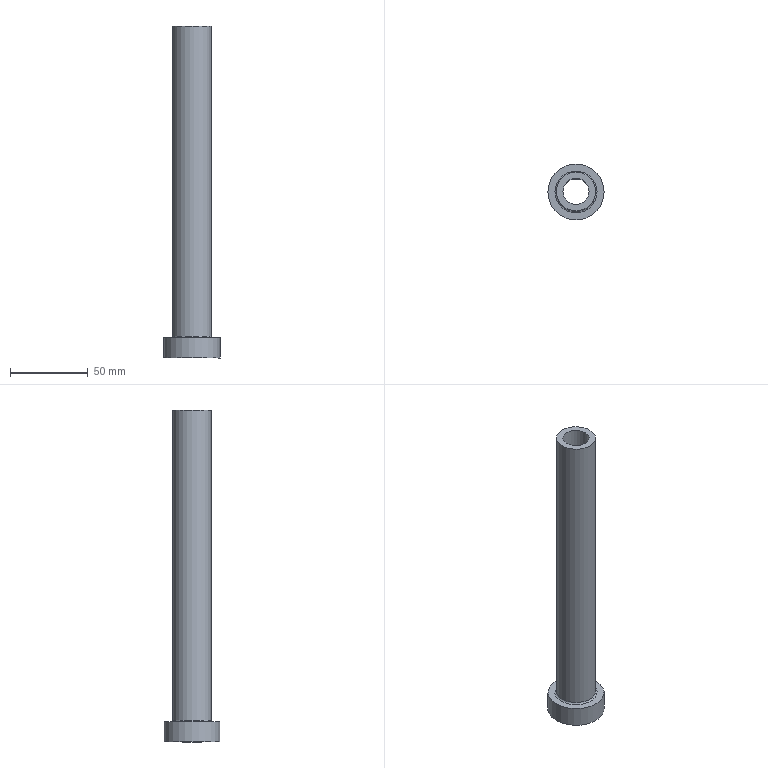Part | NX | features solid 2 | 1 solid | 7 faces | box 36 x 36 x 213 mm | volume 64208 mm3 | plane 3 | cylinder 3 | torus 1 | commonest cylinder face diameters 16.8 x1 25 x1 36 x1
STEP:
#1=CARTESIAN_POINT('',(-191.5,-358.5,175.));
#2=VERTEX_POINT('',#1);
#3=CARTESIAN_POINT('',(-205.,-358.5,175.));
#4=DIRECTION('',(0.,0.,1.));
#5=DIRECTION('',(1.,0.,0.));
#6=AXIS2_PLACEMENT_3D('',#3,#4,#5);
#7=CIRCLE('',#6,13.5);
#8=EDGE_CURVE('',#2,#2,#7,.T.);
#9=ORIENTED_EDGE('',*,*,#8,.F.);
#10=EDGE_LOOP('',(#9));
#11=FACE_BOUND('',#10,.T.);
#12=CARTESIAN_POINT('',(-223.,-358.5,175.));
#13=VERTEX_POINT('',#12);
#14=CARTESIAN_POINT('',(-205.,-358.5,175.));
#15=DIRECTION('',(0.,0.,-1.));
#16=DIRECTION('',(-1.,0.,0.));
#17=AXIS2_PLACEMENT_3D('',#14,#15,#16);
#18=CIRCLE('',#17,18.);
#19=EDGE_CURVE('',#13,#13,#18,.T.);
#20=ORIENTED_EDGE('',*,*,#19,.F.);
#21=EDGE_LOOP('',(#20));
#22=FACE_BOUND('',#21,.T.);
#23=CARTESIAN_POINT('',(-205.,-358.5,175.));
#24=DIRECTION('',(0.,0.,-1.));
#25=DIRECTION('',(1.,0.,0.));
#26=AXIS2_PLACEMENT_3D('',#23,#24,#25);
#27=PLANE('',#26);
#28=ADVANCED_FACE('',(#11,#22),#27,.F.);
#29=CARTESIAN_POINT('',(-196.6,-358.5,162.));
#30=VERTEX_POINT('',#29);
#31=CARTESIAN_POINT('',(-205.,-358.5,162.));
#32=DIRECTION('',(0.,0.,1.));
#33=DIRECTION('',(1.,0.,0.));
#34=AXIS2_PLACEMENT_3D('',#31,#32,#33);
#35=CIRCLE('',#34,8.4);
#36=EDGE_CURVE('',#30,#30,#35,.T.);
#37=ORIENTED_EDGE('',*,*,#36,.T.);
#38=EDGE_LOOP('',(#37));
#39=FACE_BOUND('',#38,.T.);
#40=CARTESIAN_POINT('',(-223.,-358.5,162.));
#41=VERTEX_POINT('',#40);
#42=CARTESIAN_POINT('',(-205.,-358.5,162.));
#43=DIRECTION('',(0.,0.,-1.));
#44=DIRECTION('',(-1.,0.,0.));
#45=AXIS2_PLACEMENT_3D('',#42,#43,#44);
#46=CIRCLE('',#45,18.);
#47=EDGE_CURVE('',#41,#41,#46,.T.);
#48=ORIENTED_EDGE('',*,*,#47,.T.);
#49=EDGE_LOOP('',(#48));
#50=FACE_BOUND('',#49,.T.);
#51=CARTESIAN_POINT('',(-205.,-358.5,162.));
#52=DIRECTION('',(0.,0.,-1.));
#53=DIRECTION('',(1.,0.,0.));
#54=AXIS2_PLACEMENT_3D('',#51,#52,#53);
#55=PLANE('',#54);
#56=ADVANCED_FACE('',(#39,#50),#55,.T.);
#57=ORIENTED_EDGE('',*,*,#19,.T.);
#58=EDGE_LOOP('',(#57));
#59=FACE_BOUND('',#58,.T.);
#60=ORIENTED_EDGE('',*,*,#47,.F.);
#61=EDGE_LOOP('',(#60));
#62=FACE_BOUND('',#61,.T.);
#63=CARTESIAN_POINT('',(-205.,-358.5,162.));
#64=DIRECTION('',(0.,0.,1.));
#65=DIRECTION('',(-1.,0.,0.));
#66=AXIS2_PLACEMENT_3D('',#63,#64,#65);
#67=CYLINDRICAL_SURFACE('',#66,18.);
#68=ADVANCED_FACE('',(#59,#62),#67,.T.);
#69=CARTESIAN_POINT('',(-196.6,-358.5,375.));
#70=VERTEX_POINT('',#69);
#71=CARTESIAN_POINT('',(-205.,-358.5,375.));
#72=DIRECTION('',(0.,0.,1.));
#73=DIRECTION('',(1.,0.,0.));
#74=AXIS2_PLACEMENT_3D('',#71,#72,#73);
#75=CIRCLE('',#74,8.4);
#76=EDGE_CURVE('',#70,#70,#75,.T.);
#77=ORIENTED_EDGE('',*,*,#76,.F.);
#78=EDGE_LOOP('',(#77));
#79=FACE_BOUND('',#78,.T.);
#80=CARTESIAN_POINT('',(-217.5,-358.5,375.));
#81=VERTEX_POINT('',#80);
#82=CARTESIAN_POINT('',(-205.,-358.5,375.));
#83=DIRECTION('',(0.,0.,-1.));
#84=DIRECTION('',(-1.,0.,0.));
#85=AXIS2_PLACEMENT_3D('',#82,#83,#84);
#86=CIRCLE('',#85,12.5);
#87=EDGE_CURVE('',#81,#81,#86,.T.);
#88=ORIENTED_EDGE('',*,*,#87,.F.);
#89=EDGE_LOOP('',(#88));
#90=FACE_BOUND('',#89,.T.);
#91=CARTESIAN_POINT('',(-205.,-358.5,375.));
#92=DIRECTION('',(0.,0.,1.));
#93=DIRECTION('',(-1.,0.,0.));
#94=AXIS2_PLACEMENT_3D('',#91,#92,#93);
#95=PLANE('',#94);
#96=ADVANCED_FACE('',(#79,#90),#95,.T.);
#97=CARTESIAN_POINT('',(-192.5,-358.5,176.));
#98=VERTEX_POINT('',#97);
#99=CARTESIAN_POINT('',(-205.,-358.5,176.));
#100=DIRECTION('',(0.,0.,1.));
#101=DIRECTION('',(1.,0.,0.));
#102=AXIS2_PLACEMENT_3D('',#99,#100,#101);
#103=CIRCLE('',#102,12.5);
#104=EDGE_CURVE('',#98,#98,#103,.F.);
#105=ORIENTED_EDGE('',*,*,#104,.F.);
#106=EDGE_LOOP('',(#105));
#107=FACE_BOUND('',#106,.T.);
#108=ORIENTED_EDGE('',*,*,#87,.T.);
#109=EDGE_LOOP('',(#108));
#110=FACE_BOUND('',#109,.T.);
#111=CARTESIAN_POINT('',(-205.,-358.5,175.));
#112=DIRECTION('',(0.,0.,1.));
#113=DIRECTION('',(-1.,0.,0.));
#114=AXIS2_PLACEMENT_3D('',#111,#112,#113);
#115=CYLINDRICAL_SURFACE('',#114,12.5);
#116=ADVANCED_FACE('',(#107,#110),#115,.T.);
#117=ORIENTED_EDGE('',*,*,#36,.F.);
#118=EDGE_LOOP('',(#117));
#119=FACE_BOUND('',#118,.T.);
#120=ORIENTED_EDGE('',*,*,#76,.T.);
#121=EDGE_LOOP('',(#120));
#122=FACE_BOUND('',#121,.T.);
#123=CARTESIAN_POINT('',(-205.,-358.5,375.));
#124=DIRECTION('',(0.,0.,-1.));
#125=DIRECTION('',(1.,0.,0.));
#126=AXIS2_PLACEMENT_3D('',#123,#124,#125);
#127=CYLINDRICAL_SURFACE('',#126,8.4);
#128=ADVANCED_FACE('',(#119,#122),#127,.F.);
#129=ORIENTED_EDGE('',*,*,#8,.T.);
#130=EDGE_LOOP('',(#129));
#131=FACE_BOUND('',#130,.T.);
#132=ORIENTED_EDGE('',*,*,#104,.T.);
#133=EDGE_LOOP('',(#132));
#134=FACE_BOUND('',#133,.T.);
#135=CARTESIAN_POINT('',(-205.,-358.5,176.));
#136=DIRECTION('',(0.,0.,-1.));
#137=DIRECTION('',(1.,0.,0.));
#138=AXIS2_PLACEMENT_3D('',#135,#136,#137);
#139=TOROIDAL_SURFACE('',#138,13.5,1.);
#140=ADVANCED_FACE('',(#131,#134),#139,.F.);
#141=CLOSED_SHELL('',(#28,#56,#68,#96,#116,#128,#140));
#142=MANIFOLD_SOLID_BREP('',#141);
#143=(LENGTH_UNIT()NAMED_UNIT(*)SI_UNIT(.MILLI.,.METRE.));
#144=UNCERTAINTY_MEASURE_WITH_UNIT(LENGTH_MEASURE(0.00001),#143,'','');
#145=(NAMED_UNIT(*)PLANE_ANGLE_UNIT()SI_UNIT($,.RADIAN.));
#146=(NAMED_UNIT(*)SI_UNIT($,.STERADIAN.)SOLID_ANGLE_UNIT());
#147=(GEOMETRIC_REPRESENTATION_CONTEXT(3)GLOBAL_UNCERTAINTY_ASSIGNED_CONTEXT((#144))GLOBAL_UNIT_ASSIGNED_CONTEXT((#143,#145,#146))REPRESENTATION_CONTEXT('',''));
#148=ADVANCED_BREP_SHAPE_REPRESENTATION('',(#142),#147);